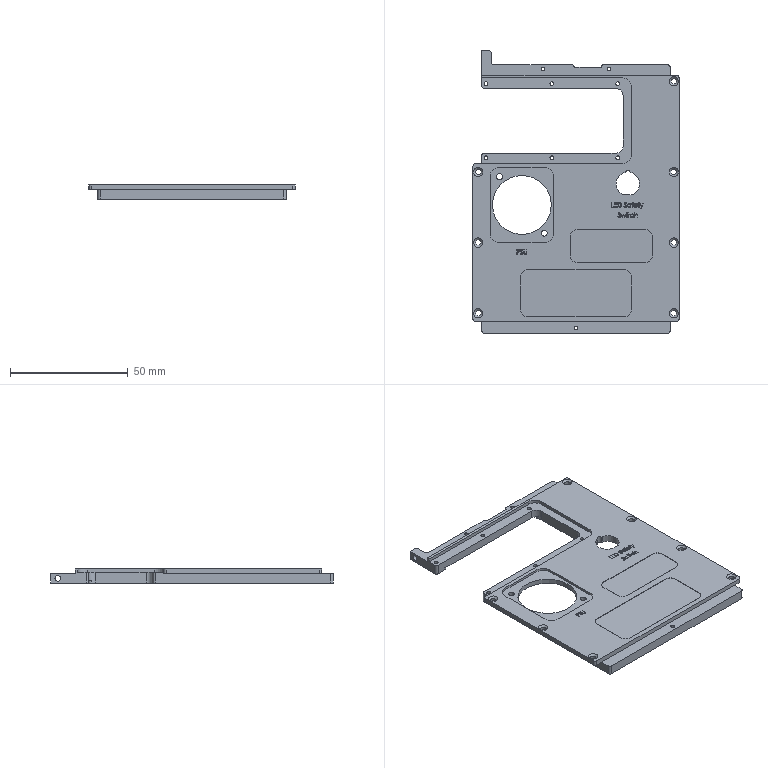NC program | NX | posted with a generic post | part box 87.5 x 120 x 6.001 mm
Lines 21 to 875 of 10039:
(ADAPTIVE_MILLING , TOOL : D6-18-D6-50-3T-ROUGH)
N40 T02 M6
N42 G53
N44 G17 G0 G90 X48.231 Y51.264 B0. C0. S6500 M3
N46 G43 Z50. H2
N48 Z-6.
N50 G94 G1 X48.234 Y51.239 Z-6.156 F3500.
N52 X48.237 Y51.214 Z-6.218
N54 X48.24 Y51.189 Z-6.263
N56 X48.243 Y51.164 Z-6.3
N58 X48.245 Y51.14 Z-6.331
N60 X48.248 Y51.115 Z-6.357
N62 X48.251 Y51.09 Z-6.38
N64 X48.254 Y51.065 Z-6.4
N66 X48.257 Y51.04 Z-6.418
N68 X48.26 Y51.015 Z-6.433
N70 X48.263 Y50.991 Z-6.447
N72 X48.266 Y50.966 Z-6.458
N74 X48.269 Y50.941 Z-6.468
N76 X48.272 Y50.916 Z-6.477
N78 X48.275 Y50.891 Z-6.484
N80 X48.277 Y50.866 Z-6.49
N82 X48.28 Y50.842 Z-6.494
N84 X48.283 Y50.817 Z-6.497
N86 X48.286 Y50.792 Z-6.499
N88 X48.289 Y50.767 Z-6.5
N90 X48.413 Y49.707
N92 G3 X48.692 Y49.265 R0.609
N94 X50.561 Y48.714 R4.722
N96 X56.014 Y48.464 R47.78
N98 G2 X60.858 Y48.431 R266.092
N100 X63.215 Y46.822 R3.486
N102 X64.391 Y43.389 R8.174
N104 X64.685 Y37.641 R45.423
N106 G1 X64.7 Y31.101
N108 X64.698 Y-44.39
N110 G2 X63.333 Y-46.758 R3.265
N112 X60.017 Y-48.071 R7.403
N114 X54.634 Y-48.425 R35.724
N116 G1 X46.714 Y-48.45
N118 X-60.638 Y-48.448
N120 G2 X-63.007 Y-47.073 R3.28
N122 X-64.322 Y-43.746 R7.447
N124 X-64.674 Y-38.363 R35.875
N126 G1 X-64.699 Y-30.563
N128 X-64.698 Y44.37
N130 G2 X-63.389 Y46.705 R3.246
N132 X-60.131 Y48.048 R7.217
N134 X-55.11 Y48.417 R32.115
N136 X-46.711 Y48.45 R653.142
N138 G1 X46.218 Y48.448
N140 G2 X49.506 Y48.064 R34.565
N142 G3 X56.918 Y47.67 R62.985
N144 G2 X59.184 Y47.6 R18.211
N146 X62.338 Y45.284 R4.681
N148 X63.573 Y41.358 R10.249
N150 X63.882 Y35.25 R51.582
N152 G1 X63.9 Y27.99
N154 X63.897 Y-42.368
N156 G2 X61.805 Y-45.898 R4.481
N158 X58.051 Y-47.25 R9.298
N160 X52.428 Y-47.62 R40.051
N162 G1 X44.388 Y-47.65
N164 X-58.572 Y-47.648
N166 G2 X-62.125 Y-45.582 R4.464
N168 X-63.511 Y-41.715 R9.344
N170 X-63.865 Y-36.271 R39.668
N172 X-63.899 Y-27.031 R690.714
N174 G1 Y42.288
N176 G2 X-61.821 Y45.884 R4.471
N178 X-58.004 Y47.256 R9.32
N180 X-52.501 Y47.616 R39.83
N182 G1 X-43.741 Y47.649
N184 X44.579 Y47.647
N186 G2 X49.672 Y47.237 R56.663
N188 G3 X57.232 Y46.862 R109.931
N190 G2 X61.401 Y44.156 R5.305
N192 X62.728 Y40.005 R11.071
N194 X63.078 Y33.659 R51.071
N196 G1 X63.1 Y26.399
N198 X63.099 Y-36.377
N200 X63.15 Y-36.998
N202 G2 X63.092 Y-41.028 R53.968
N204 X60.396 Y-45.143 R5.307
N206 X56.313 Y-46.466 R10.952
N208 X50.088 Y-46.825 R48.919
N210 G1 X42.168 Y-46.849
N212 X11.476 Y-46.85
N214 X10.999 Y-46.9
N216 X-54.442 Y-46.89
N218 G2 X-57.473 Y-46.816 R47.115
N220 X-61.37 Y-44.178 R5.29
N222 X-62.531 Y-41.145 R10.542
N224 X-63.065 Y-39.836 R4.344
N226 G1 X-63.15 Y-38.999
N228 X-63.145 Y39.222
N230 G2 X-63.008 Y41.628 R14.584
N232 X-60.283 Y45.21 R5.399
N234 X-56.24 Y46.475 R11.241
N236 G3 X-54.868 Y46.808 R4.797
N238 G1 X-54. Y46.9
N240 X48.501
N242 G2 X50.207 Y46.608 R9.102
N244 G3 X55.546 Y46.131 R38.286
N246 G2 X60.628 Y42.907 R5.952
N248 X61.938 Y38.495 R12.488
N250 X62.282 Y31.488 R60.228
N252 G1 X62.299 Y24.228
N254 X62.304 Y-34.388
N256 G3 X62.596 Y-34.928 R1.144
N258 G2 X63.1 Y-36.39 R4.185
N260 G1 X63.095 Y-36.33
N262 X62.934 Y-35.679
N264 G3 X62.596 Y-34.928 R4.351
N266 G2 X62.073 Y-33.687 R2.244
N268 X61.839 Y-29.756 R28.017
N270 G1 X61.819 Y-24.746
N272 X61.818 Y26.614
N274 G3 X61.664 Y35.971 R171.609
N276 X60.881 Y40.755 R19.457
N278 X58.658 Y44.117 R6.781
N280 X55.333 Y45.433 R7.527
N282 X51.211 Y45.987 R223.313
N284 G1 X50.951 Y46.099
N286 G3 X49.455 Y46.78 R4.647
N288 G2 X51.231 Y45.865 R4.245
N290 G3 X53.493 Y45.066 R7.668
N292 G2 X56.36 Y44.203 R14.581
N294 X59.706 Y40.547 R6.854
N296 X60.775 Y35.701 R16.143
N298 X61.013 Y27.607 R99.409
N300 G1 X61.019 Y21.967
N302 X61.02 Y-25.624
N304 G3 X61.162 Y-32.167 R87.18
N306 X61.393 Y-33.54 R6.272
N308 X62.085 Y-34.225 R3.54
N310 G1 X62.332 Y-34.565
N312 G3 X61.504 Y-33.7 R3.765
N314 G2 X61.02 Y-32.773 R1.83
N316 X60.61 Y-29.385 R15.183
N318 X60.539 Y-22.286 R254.423
N320 G1 X60.537 Y25.174
N322 G3 X60.373 Y34.351 R162.186
N324 X59.573 Y39.192 R19.888
N326 X56.631 Y43.154 R7.086
N328 X53.72 Y44.413 R13.134
N330 G2 X51.94 Y45.091 R12.871
N332 X51.597 Y45.512 R2.369
N334 G1 X51.108 Y45.956
N336 G2 X51.994 Y44.959 R3.712
N338 G3 X53.572 Y43.88 R5.597
N340 G2 X56.246 Y42.214 R13.059
N342 X58.804 Y38.005 R8.749
N344 X59.595 Y32.675 R23.4
N346 X59.738 Y22.838 R205.782
N348 G1 X59.739 Y-21.966
N350 G3 X59.86 Y-29.751 R139.122
N352 X60.412 Y-32.849 R10.652
N354 X60.689 Y-33.209 R0.809
N356 G1 X61.44 Y-33.643
N358 X60.577 Y-33.155
N360 G2 X59.845 Y-31.806 R2.823
N362 X59.35 Y-28.049 R16.534
N364 X59.259 Y-19.706 R223.119
N366 G1 X59.257 Y23.254
N368 G3 X59.084 Y32.851 R164.747
N370 X58.241 Y37.867 R20.503
N372 X56.79 Y40.656 R10.234
N374 G1 X56.739 Y40.801
N376 X56.245 Y41.587
N378 X55.587 Y42.245
N380 G3 X53.523 Y43.401 R20.997
N382 G2 X52.406 Y44.164 R4.996
N384 G1 X52.106 Y44.804
N386 X51.966 Y44.999
N388 G2 X52.344 Y44.26 R2.906
N390 G3 X53.26 Y43.142 R2.123
N392 X53.923 Y43.046 R6.592
N394 G1 X54.801 Y42.739
N396 X53.923 Y43.046
N398 G2 X53.122 Y43.167 R3.302
N400 X52.456 Y44.005 R0.968
N402 G3 X52.669 Y43.365 R1.378
N404 X53.27 Y43.12 R0.812
N406 G1 X53.923 Y43.046
N408 X54.801 Y42.739
N410 X55.587 Y42.245
N412 X56.245 Y41.587
N414 X56.739 Y40.801
N416 G2 X57.148 Y39.32 R5.513
N418 X58.384 Y29.657 R41.743
N420 X58.459 Y19.698 R459.539
N422 G1 X58.46 Y-21.064
N424 G3 X58.633 Y-28.817 R106.579
N426 X59.32 Y-32.159 R11.11
N428 X59.842 Y-32.921 R1.567
N430 G1 X60.689 Y-33.209
N432 X59.806 Y-32.924
N434 G2 X58.927 Y-31.785 R2.327
N436 X58.197 Y-28.457 R11.099
N438 X57.986 Y-21.796 R79.421
N440 G1 X57.979 Y-16.526
N442 Y36.514
N444 X57.98 Y36.547
N446 X58.083 Y38.365
N448 X58.118 Y38.845 Z-6.459
N450 G2 X58.584 Y39.302 Z-6.4 R0.606
N452 X59.297 Y38.797 R0.6 F15000.
N454 G1 X59.332 Y38.56
N456 X59.355 Y38.322
N458 G2 X58.633 Y37.756 R0.6
N460 X58.161 Y38.439 Z-6.478 R0.607 F3500.
N462 G1 X58.18 Y38.694 Z-6.5
N464 X58.261 Y39.767
N466 G3 X57.066 Y39.745 R-0.6
N468 G1 X57.15 Y38.999
N470 X57.157 Y10.899
N472 X57.179 Y2.619
N474 X57.18 Y-18.666
N476 G3 X57.348 Y-27.396 R136.933
N478 X58.09 Y-31.365 R14.301
N480 X58.95 Y-32.758 R3.687
N482 G1 X59.224 Y-32.874
N484 X59.863 Y-32.941
N486 G2 X58.964 Y-32.811 R3.687
N488 X57.86 Y-31.486 R2.814
N490 X57.15 Y-29.077 R9.496
N492 G1 Y-1.501
N494 X56.854 Y0.539
N496 G2 X56.704 Y5.446 R61.609
N498 G1 X56.696 Y9.702
N500 X57.034 Y10.587
N502 X57.15 Y11.499
N504 X57.034 Y10.587
N506 G2 X56.441 Y9.192 R40.775
N508 G3 X56.15 Y7.816 R9.32
N510 G1 X56.164 Y1.087
N512 X56.276 Y0.839
N514 X56.693 Y0.268
N516 X57.034 Y-0.587
N518 X56.693 Y0.268
N520 X56.276 Y0.839
N522 G2 X56.15 Y1.222 R0.665
N524 X56.166 Y8.856 R560.007
N526 X56.276 Y9.161 R0.851
N528 G1 X56.665 Y9.694
N530 G3 X56.197 Y9.012 R6.747
N532 X56.15 Y8.598 R1.645
N534 X56.407 Y8.105 R0.602
N536 G1 X56.662 Y7.928
N538 X57.624 Y7.259 Z-6.4
N540 X57.776 Y7.153 F15000.
N542 X57.906 Y7.02
N544 G2 X58.014 Y6.733 R0.64
N546 G1 X58.306 Y3.925
N548 X58.586 Y1.116
N550 G2 X58.934 Y-6.398 R88.816
N552 G1 X59.014 Y-27.212
N554 G2 X58.741 Y-27.718 R0.602
N556 G1 X58.623 Y-27.795
N558 X57.64 Y-28.433 Z-6.5 F3500.
N560 X57.345 Y-28.634
N562 G3 X57.15 Y-29.077 R0.605
N564 X57.191 Y-30.784 R11.965
N566 X58.2 Y-32.731 R3.335
N568 X58.535 Y-32.85 R1.13
N570 G1 X59.12 Y-32.863
N572 X58.415 Y-32.85
N574 G2 X57.456 Y-32.09 R1.629
N576 X57.15 Y-31.425 R1.686
N578 G1 Y-30.405
N580 X57.165 Y-31.843
N582 G3 X57.762 Y-32.788 R1.334
N584 X58.473 Y-32.85 R1.823
N586 G2 X57.738 Y-32.818 R2.723
N588 X57.15 Y-32.091 R0.951
N590 G1 Y-31.671
N592 G3 X57.172 Y-32.368 R13.47
N594 X57.98 Y-32.85 R0.711
N596 G2 X59.863 Y-32.941 R9.94
N598 X62.085 Y-34.225 R4.477
N600 G1 X62.596 Y-34.928
N602 G2 X62.934 Y-35.679 R4.351
N604 X63.15 Y-36.998 R4.495
N606 X63.121 Y-40.429 R56.537
N608 G1 X63.034 Y-40.847
N610 X62.669 Y-41.673
N612 G2 X57.098 Y-45.279 R9.596
N614 X51.509 Y-45.953 R27.376
N616 X40.41 Y-46.049 R341.091
N618 G1 X13.642 Y-46.053
N620 X13.418 Y-46.118
N622 G2 X11.868 Y-46.808 R4.677
N624 G1 X11.45 Y-46.852
N626 X11.868 Y-46.808
N628 G3 X13.5 Y-46.064 R4.808
N630 G2 X15.554 Y-45.685 R6.518
N632 X23.343 Y-45.569 R137.9
N634 G1 X43.443 Y-45.567
N636 G3 X52.62 Y-45.396 R154.11
N638 X57.687 Y-44.502 R19.437
N640 X60.288 Y-43.143 R10.269
N642 G2 X60.788 Y-43.05 R2.631
N644 G3 X62.166 Y-42.287 R3.662
N646 G2 X60.788 Y-43.05 R3.662
N648 G3 X58.112 Y-43.601 R14.811
N650 G2 X50.162 Y-44.672 R34.432
N652 X38.643 Y-44.769 R372.365
N654 G1 X22.226 Y-44.77
N656 G3 X15.809 Y-44.918 R82.244
N658 X14.414 Y-45.172 R4.888
N660 X14.097 Y-45.512 R1.186
N662 G1 X13.451 Y-46.099
N664 G3 X14.34 Y-45.182 R4.391
N666 G2 X15.957 Y-44.605 R3.761
N668 X20.792 Y-44.309 R32.801
N670 G1 X25.563 Y-44.289
N672 X41.583 Y-44.287
N674 G3 X51.72 Y-44.094 R167.09
N676 X57.841 Y-43.15 R34.625
N678 G1 X59.999
N680 X54.121
N682 G2 X41.49 Y-43.484 R181.661
N684 G1 X36.93 Y-43.489
N686 X24.626 Y-43.49
N688 G3 X17.719 Y-43.653 R91.021
N690 X15.006 Y-44.224 R8.614
N692 X14.606 Y-44.804 R1.055
N694 G1 X14.291 Y-45.242
N696 G3 X14.791 Y-44.381 R2.588
N698 G2 X15.973 Y-43.663 R2.371
N700 X19.584 Y-43.119 R14.315
N702 X26.884 Y-43.009 R160.409
N704 G1 X39.723 Y-43.007
N706 X44.02 Y-43.008
N708 G3 X44.997 Y-43.15 R2.845
N710 G1 X54.177
N712 X44.882 Y-43.148
N714 G2 X43.319 Y-42.795 R5.248
N716 G3 X40.388 Y-42.327 R10.952
N718 X31.281 Y-42.21 R186.605
N720 X20.46 Y-42.301 R291.363
N722 X17.504 Y-42.612 R17.656
N724 G2 X16.214 Y-43.091 R4.318
N726 G3 X15.15 Y-43.553 R2.533
N728 X14.956 Y-44.005 R0.867
N730 G1 X14.787 Y-44.389
N732 G3 X15.016 Y-43.71 R2.058
N734 G2 X15.688 Y-43.13 R1.073
N736 G1 X16.361 Y-43.06
N738 G3 X15.437 Y-43.177 R16.635
N740 X15.003 Y-43.774 R0.694
N742 G2 X15.17 Y-43.364 R0.824
N744 X15.596 Y-43.14 R0.696
N746 G3 X17.803 Y-42.447 R4.335
N748 G2 X20.506 Y-41.904 R9.013
N750 X27.605 Y-41.731 R97.498
N752 X39.377 Y-41.815 R355.937
N754 X42.244 Y-42.127 R16.477
N756 G3 X43.374 Y-42.818 R12.847
N758 G1 X42.534 Y-42.338
N760 G3 X40.954 Y-41.485 R3.086
N762 X36.954 Y-41.016 R19.258
N764 X22.147 Y-41.03 R257.397
N766 X18.927 Y-41.44 R14.877
N768 X18.58 Y-41.781 R0.993
N770 G1 X17.936 Y-42.36
N772 X17.676 Y-42.51
N774 G3 X18.775 Y-41.514 R3.554
N776 G2 X20.23 Y-40.904 R3.309
N778 X24.668 Y-40.5 R24.661
N780 X37.195 Y-40.564 R219.745
N782 X40.993 Y-41.109 R15.928
N784 X41.692 Y-41.47 R1.406
N786 G3 X42.266 Y-42.087 R2.592
N788 G2 X41.559 Y-41.269 R2.636
N790 G3 X39.955 Y-40.376 R3.533
N792 X35.84 Y-39.781 R17.814
N794 X23.256 Y-39.785 R145.835
N796 X19.768 Y-40.373 R12.961
N798 X19.265 Y-40.727 R0.871
N800 G2 X18.772 Y-41.519 R3.182
N802 G3 X19.349 Y-40.568 R4.184
N804 G2 X20.821 Y-39.798 R3.186
N806 X24.842 Y-39.271 R18.285
N808 X36.417 Y-39.362 R117.882
N810 X40.167 Y-40.06 R14.116
N812 X41.165 Y-40.614 R2.714
N814 G3 X41.56 Y-41.27 R8.46
N816 G2 X41.14 Y-40.49 R3.083
N818 G3 X39.608 Y-39.399 R3.214
N820 X35.701 Y-38.607 R14.015
N822 X23.729 Y-38.582 R85.658
N824 X20.371 Y-39.297 R11.492
N826 X19.599 Y-39.812 R1.641
N828 G1 X19.312 Y-40.632
N830 X19.593 Y-39.752
N832 G2 X20.851 Y-38.85 R2.721
N834 X24.416 Y-38.111 R12.482
N836 X35.88 Y-38.174 R74.25
N838 X39.713 Y-39.055 R12.83
N840 X40.914 Y-39.869 R3.193
N842 G1 X41.21 Y-40.637
N844 G3 X40.853 Y-39.633 R45.482
N846 X39.288 Y-38.382 R3.471
N848 X35.507 Y-37.444 R12.742
N850 X24.245 Y-37.378 R59.726
N852 X20.77 Y-38.224 R11.333
N854 X19.715 Y-38.972 R2.762
N856 G1 X19.631 Y-39.184
N858 X19.528 Y-39.957
N860 X19.66 Y-39.007
N862 G2 X20.804 Y-37.942 R2.468
N864 X24.18 Y-36.985 R10.144
N866 X32.363 Y-36.749 R50.589
N868 X37.677 Y-37.408 R25.735
N870 X40.439 Y-38.737 R6.625
N872 X40.894 Y-39.37 R1.327
N874 G1 X40.956 Y-39.907
N876 G3 X40.795 Y-38.918 R3.767
N878 X39.242 Y-37.444 R3.461
N880 X35.485 Y-36.312 R11.647
N882 X24.359 Y-36.223 R44.377
N884 X20.779 Y-37.285 R10.443
N886 X19.714 Y-38.183 R2.867
N888 G1 X19.65 Y-38.417
N890 X19.642 Y-39.105
N892 X19.65 Y-38.297
N894 G2 X20.472 Y-37.218 R1.997
N896 X23.495 Y-35.987 R7.807
N898 X29.528 Y-35.476 R29.768
N900 X36.455 Y-36.057 R33.73
N902 X39.828 Y-37.413 R9.077
N904 X40.825 Y-38.516 R2.76
N906 G1 X40.871 Y-39.178
N908 X40.832 Y-38.305
N910 G3 X39.677 Y-36.794 R2.916
N912 X36.154 Y-35.331 R9.302
N914 X28.91 Y-34.725 R32.438
N916 X23.11 Y-35.364 R24.805
N918 X20.146 Y-36.79 R7.173
N920 X19.653 Y-37.496 R1.27
N922 G1 X19.65 Y-38.305
N924 G2 X19.683 Y-37.265 R4.687
N926 X20.95 Y-35.909 R2.973
N928 X24.69 Y-34.636 R10.371
N930 X35.835 Y-34.829 R33.454
N932 X39.576 Y-36.305 R10.218
N934 X40.813 Y-37.65 R3.715
N936 X40.85 Y-38.426 R2.528
N938 G3 X40.814 Y-37.374 R5.174
N940 X39.521 Y-35.713 R3.351
N942 X35.731 Y-34.132 R10.121
N944 X24.393 Y-33.965 R30.581
N946 X20.67 Y-35.391 R9.872
N948 X19.699 Y-36.362 R3.154
N950 G1 X19.65 Y-36.566
N952 Y-37.406
N954 Y-36.446
N956 G2 X20.498 Y-35.231 R2.294
N958 X23.675 Y-33.737 R8.186
N960 X30.207 Y-33.092 R24.764
N962 X36.723 Y-33.965 R24.498
N964 X40.051 Y-35.728 R8.366
N966 X40.832 Y-36.804 R3.013
N968 G1 X40.85 Y-37.635
N970 G3 X40.818 Y-36.46 R7.08
N972 X39.564 Y-34.747 R3.405
N974 X35.736 Y-33.024 R10.076
N976 X24.369 Y-32.85 R27.35
N978 X20.664 Y-34.37 R9.946
N980 X19.695 Y-35.375 R3.223
N982 G1 X19.65 Y-35.565
N984 Y-36.465
N986 G2 X19.679 Y-35.312 R6.194
N988 X20.974 Y-33.832 R3.247
N990 X24.884 Y-32.339 R10.652
N992 X35.968 Y-32.655 R26.506
N994 X39.696 Y-34.417 R9.975
N996 X40.83 Y-35.828 R3.731
N998 X40.85 Y-36.726 R10.285
N1000 G3 X40.832 Y-35.532 R38.393
N1002 X39.571 Y-33.73 R3.464
N1004 X35.749 Y-31.918 R10.129
N1006 X24.229 Y-31.765 R25.111
N1008 X20.546 Y-33.414 R9.695
N1010 X19.696 Y-34.341 R3.276
N1012 G1 X19.65 Y-34.536
N1014 Y-35.496
N1016 Y-34.416
N1018 G2 X20.572 Y-33.086 R2.532
N1020 X24.102 Y-31.4 R9.046
N1022 X32.133 Y-30.862 R23.817
N1024 X37.833 Y-32.232 R17.632
N1026 X40.53 Y-34.278 R6.76
N1028 X40.85 Y-34.936 R1.562
N1030 G1 Y-35.656
N1032 G3 X40.831 Y-34.516 R20.118
N1034 X39.585 Y-32.697 R3.544
N1036 X35.719 Y-30.796 R10.231
N1038 X24.138 Y-30.672 R23.615
N1040 X20.496 Y-32.394 R9.604
N1042 X19.693 Y-33.299 R3.197
N1044 G1 X19.65 Y-33.485
N1046 Y-34.445
N1048 Y-33.365
N1050 G2 X20.584 Y-32.006 R2.605
N1052 X24.078 Y-30.289 R9.168
N1054 X32.45 Y-29.747 R22.78
N1056 X38.023 Y-31.244 R16.631
N1058 X40.591 Y-33.335 R6.599
N1060 X40.85 Y-33.91 R1.383
N1062 G1 Y-34.69
N1064 G3 X40.833 Y-33.491 R51.415
N1066 X39.6 Y-31.648 R3.578
N1068 X35.695 Y-29.674 R10.325
N1070 X24.151 Y-29.55 R22.636
N1072 X20.512 Y-31.304 R9.764
N1074 X19.69 Y-32.239 R3.185
N1076 G1 X19.65 Y-32.416
N1078 Y-33.376
N1080 Y-32.296
N1082 G2 X20.501 Y-31.001 R2.56
N1084 X23.899 Y-29.224 R8.876
N1086 X32.167 Y-28.574 R21.641
N1088 X37.97 Y-30.129 R16.77
N1090 X40.597 Y-32.293 R6.734
N1092 X40.85 Y-32.859 R1.453
N1094 G1 Y-33.639
N1096 G3 X40.811 Y-32.334 R6.822
N1098 X39.407 Y-30.407 R3.99
N1100 X35.161 Y-28.405 R11.249
N1102 X24.053 Y-28.46 R21.904
N1104 X20.404 Y-30.31 R9.59
N1106 X19.673 Y-31.21 R2.503
N1108 X19.65 Y-32.355 R8.524
N1110 G1 Y-31.215
N1112 G2 X20.503 Y-29.908 R2.574
N1114 X23.965 Y-28.085 R9.043
N1116 X32.704 Y-27.498 R21.282
N1118 X38.364 Y-29.247 R15.539
N1120 X40.704 Y-31.402 R6.211
N1122 X40.85 Y-31.797 R1.29
N1124 G1 Y-32.577
N1126 G3 X40.816 Y-31.287 R7.102
N1128 X39.462 Y-29.366 R3.941
N1130 X35.302 Y-27.321 R11.08
N1132 X24.006 Y-27.354 R21.313
N1134 X20.364 Y-29.254 R9.473
N1136 X19.673 Y-30.123 R2.428
N1138 X19.65 Y-31.266 R6.615
N1140 G1 Y-30.126
N1142 G2 X20.543 Y-28.774 R2.65
N1144 X24.146 Y-26.91 R9.346
N1146 X36.412 Y-27.247 R20.887
N1148 X40.017 Y-29.416 R9.468
N1150 X40.84 Y-30.641 R3.317
N1152 G1 X40.85 Y-31.551
N1154 G3 X40.817 Y-30.205 R8.379
N1156 X39.502 Y-28.305 R3.934
N1158 X35.343 Y-26.21 R11.011
N1160 X23.958 Y-26.248 R20.87
N1162 X20.394 Y-28.127 R9.546
N1164 X19.671 Y-29.032 R2.464
N1166 X19.65 Y-30.17 R8.387
N1168 G1 Y-29.03
N1170 G2 X20.581 Y-27.635 R2.706
N1172 X24.206 Y-25.77 R9.544
N1174 X36.457 Y-26.146 R20.518
N1176 X40.05 Y-28.357 R9.43
N1178 X40.833 Y-29.524 R3.706
N1180 G1 X40.85 Y-30.469
N1182 G3 X40.817 Y-29.118 R8.662
N1184 X39.458 Y-27.165 R4.006
N1186 X35.179 Y-25.04 R11.266
N1188 X23.908 Y-25.142 R20.544
N1190 X20.371 Y-27.041 R9.482
N1192 X19.685 Y-27.881 R2.891
N1194 G1 X19.65 Y-28.053
N1196 Y-29.073
N1198 X19.654 Y-27.873
N1200 G2 X20.758 Y-26.371 R3.097
N1202 X24.748 Y-24.494 R10.455
N1204 X36.398 Y-25.006 R20.364
N1206 X40.057 Y-27.265 R9.508
N1208 X40.835 Y-28.433 R3.637
N1210 G1 X40.85 Y-29.37
N1212 G3 X40.818 Y-28.022 R7.93
N1214 X39.49 Y-26.087 R3.994
N1216 X35.224 Y-23.928 R11.2
N1218 X23.858 Y-24.036 R20.277
N1220 X20.293 Y-26.003 R9.338
N1222 X19.672 Y-26.813 R2.301
N1224 X19.65 Y-27.953 R7.306
N1226 G1 Y-26.813
N1228 G2 X20.587 Y-25.408 R2.744
N1230 X24.323 Y-23.488 R9.736
N1232 X36.458 Y-23.908 R20.066
N1234 X40.035 Y-26.135 R9.555
N1236 X40.841 Y-27.355 R3.307
N1238 G1 X40.85 Y-28.259
N1240 G3 X40.816 Y-26.907 R8.224
N1242 X39.434 Y-24.927 R4.08
N1244 X35.116 Y-22.772 R11.408
N1246 X23.752 Y-22.949 R20.041
N1248 X20.313 Y-24.87 R9.296
N1250 X19.668 Y-25.715 R2.26
N1252 X19.65 Y-26.852 R19.118
N1254 G1 X19.654 Y-25.652
N1256 G2 X20.764 Y-24.137 R3.124
N1258 X24.86 Y-22.214 R10.616
N1260 X36.443 Y-22.781 R19.97
N1262 X40.083 Y-25.076 R9.496
N1264 X40.845 Y-26.274 R3.031
N1266 G1 X40.85 Y-27.161
N1268 G3 X40.817 Y-25.805 R8.663
N1270 X39.446 Y-23.822 R4.071
N1272 X35.163 Y-21.66 R11.356
N1274 X23.808 Y-21.806 R19.944
N1276 X20.256 Y-23.808 R9.27
N1278 X19.671 Y-24.587 R2.214
N1280 X19.65 Y-25.725 R7.885
N1282 G1 Y-24.585
N1284 G2 X20.503 Y-23.253 R2.649
N1286 X24.059 Y-21.32 R9.339
N1288 X36.599 Y-21.719 R19.674
N1290 X40.13 Y-24.016 R9.299
N1292 X40.843 Y-25.152 R3.068
N1294 G1 X40.85 Y-26.051
N1296 G3 X40.814 Y-24.684 R8.242
N1298 X39.515 Y-22.769 R4.002
N1300 X35.313 Y-20.579 R11.1
N1302 X23.756 Y-20.699 R19.797
N1304 X20.342 Y-22.611 R9.327
N1306 X19.683 Y-23.433 R2.828
N1308 X19.65 Y-24.619 R6.036
N1310 G2 X19.678 Y-23.341 R7.754
N1312 X20.954 Y-21.747 R3.538
N1314 X25.324 Y-19.847 R11.411
N1316 X36.447 Y-20.536 R19.78
N1318 X40.084 Y-22.848 R9.552
N1320 X40.839 Y-24.013 R3.404
N1322 G1 X40.85 Y-24.928
N1324 G3 X40.812 Y-23.557 R7.702
N1326 X39.402 Y-21.55 R4.163
N1328 X34.951 Y-19.349 R11.626
N1330 X23.703 Y-19.593 R19.701
N1332 X20.288 Y-21.54 R9.23
N1334 X19.671 Y-22.355 R2.328
N1336 X19.65 Y-23.493 R8.075
N1338 G1 Y-22.353
N1340 G2 X20.597 Y-20.926 R2.782
N1342 X24.303 Y-18.994 R9.796
N1344 X36.542 Y-19.449 R19.573
N1346 X40.103 Y-21.751 R9.443
N1348 X40.837 Y-22.892 R3.502
N1350 G1 X40.85 Y-23.815
N1352 G3 X40.816 Y-22.457 R8.58
N1354 X39.47 Y-20.488 R4.068
N1356 X35.155 Y-18.281 R11.347
N1358 X23.704 Y-18.468 R19.626
N1360 X20.197 Y-20.509 R9.126
N1362 X19.66 Y-21.279 R1.837
N1364 G1 X19.65 Y-22.369
N1366 Y-21.229
N1368 G2 X20.503 Y-19.892 R2.66
N1370 X24.121 Y-17.925 R9.431
N1372 X36.594 Y-18.345 R19.464
N1374 X40.092 Y-20.618 R9.447
N1376 X40.842 Y-21.794 R3.243
N1378 G1 X40.85 Y-22.694
N1380 G3 X40.814 Y-21.327 R8.096
N1382 X39.513 Y-19.406 R4.038
N1384 X35.307 Y-17.201 R11.143
N1386 X23.65 Y-17.362 R19.54
N1388 X20.257 Y-19.331 R9.087
N1390 X19.667 Y-20.128 R2.129
N1392 X19.65 Y-21.258 R36.771
N1394 G2 X19.678 Y-19.979 R7.768
N1396 X20.921 Y-18.407 R3.518
N1398 X25.176 Y-16.504 R11.23
N1400 X36.486 Y-17.178 R19.568
N1402 X40.081 Y-19.485 R9.551
N1404 X40.838 Y-20.653 R3.467
N1406 G1 X40.85 Y-21.571
N1408 G3 X40.817 Y-20.218 R8.642
N1410 X39.475 Y-18.249 R4.087
N1412 X35.101 Y-16.013 R11.394
N1414 X23.651 Y-16.236 R19.514
N1416 X20.218 Y-18.244 R9.074
N1418 X19.671 Y-18.992 R2.167
N1420 X19.65 Y-20.13 R8.745
N1422 G2 X19.678 Y-18.852 R7.448
N1424 X20.922 Y-17.282 R3.518
N1426 X25.28 Y-15.353 R11.318
N1428 X36.539 Y-16.074 R19.51
N1430 X40.103 Y-18.386 R9.473
N1432 X40.837 Y-19.531 R3.5
N1434 G1 X40.85 Y-20.453
N1436 G3 X40.816 Y-19.095 R8.652
N1438 X39.475 Y-17.124 R4.075
N1440 X35.151 Y-14.902 R11.36
N1442 X23.706 Y-15.091 R19.515
N1444 X20.226 Y-17.112 R9.166
N1446 X19.664 Y-17.895 R1.987
N1448 G1 X19.65 Y-19.005
N1450 Y-17.865
N1452 G2 X20.548 Y-16.478 R2.726
N1454 X24.169 Y-14.532 R9.593
N1456 X36.644 Y-14.991 R19.339
N1458 X40.094 Y-17.253 R9.4
N1460 X40.842 Y-18.431 R3.226
N1462 G1 X40.85 Y-19.331
N1464 G3 X40.814 Y-17.964 R8.234
N1466 X39.438 Y-15.966 R4.136
N1468 X35.048 Y-13.746 R11.53
N1470 X23.706 Y-13.966 R19.499
N1472 X20.235 Y-15.978 R9.179
N1474 X19.666 Y-16.76 R2.063
N1476 G1 X19.65 Y-17.884
N1478 G2 X19.676 Y-16.611 R8.297
N1480 X20.922 Y-15.033 R3.512
N1482 X25.281 Y-13.1 R11.334
N1484 X36.591 Y-13.843 R19.433
N1486 X40.116 Y-16.154 R9.384
N1488 X40.84 Y-17.297 R3.32
N1490 G1 X40.85 Y-18.205
N1492 G3 X40.816 Y-16.848 R8.65
N1494 X39.51 Y-14.908 R4.036
N1496 X35.201 Y-12.664 R11.243
N1498 X23.652 Y-12.859 R19.44
N1500 X20.198 Y-14.891 R9.05
N1502 X19.663 Y-15.65 R1.898
N1504 G1 X19.65 Y-16.754
N1506 Y-15.614
N1508 G2 X20.528 Y-14.247 R2.73
N1510 X24.17 Y-12.28 R9.567
N1512 X36.59 Y-12.717 R19.332
N1514 X40.171 Y-15.093 R9.309
N1516 X40.838 Y-16.166 R3.326
N1518 G1 X40.85 Y-17.082
N1520 G3 X40.816 Y-15.723 R8.611
N1522 X39.473 Y-13.749 R4.098
N1524 X35.098 Y-11.508 R11.411
N1526 X23.652 Y-11.733 R19.432
N1528 X20.22 Y-13.743 R9.096
N1530 X19.671 Y-14.493 R2.179
N1532 X19.65 Y-15.631 R8.478
N1534 G1 Y-14.491
N1536 G2 X20.597 Y-13.058 R2.793
N1538 X24.32 Y-11.108 R9.845
N1540 X36.643 Y-11.613 R19.311
N1542 X40.193 Y-13.994 R9.219
N1544 X40.847 Y-15.091 R2.758
N1546 G1 X40.85 Y-15.958
N1548 G3 X40.816 Y-14.597 R8.548
N1550 X39.473 Y-12.624 R4.087
N1552 X35.141 Y-10.395 R11.374
N1554 X23.707 Y-10.588 R19.45
N1556 X20.227 Y-12.611 R9.183
N1558 X19.664 Y-13.394 R1.999
N1560 G1 X19.65 Y-14.506
N1562 Y-13.366
N1564 G2 X20.548 Y-11.978 R2.729
N1566 X24.172 Y-10.028 R9.595
N1568 X36.643 Y-10.487 R19.277
N1570 X40.092 Y-12.753 R9.415
N1572 X40.841 Y-13.932 R3.268
N1574 G1 X40.85 Y-14.832
N1576 G3 X40.814 Y-13.465 R8.186
N1578 X39.436 Y-11.465 R4.146
N1580 X35.046 Y-9.241 R11.539
N1582 X23.707 Y-9.462 R19.447
N1584 X20.235 Y-11.477 R9.19
N1586 X19.666 Y-12.26 R2.068
N1588 G1 X19.65 Y-13.384
N1590 G2 X19.676 Y-12.111 R8.301
N1592 X20.923 Y-10.531 R3.516
N1594 X25.282 Y-8.595 R11.361
N1596 X36.59 Y-9.339 R19.386
N1598 X40.116 Y-11.653 R9.407
N1600 X40.84 Y-12.798 R3.336
N1602 G1 X40.85 Y-13.706
N1604 G3 X40.816 Y-12.348 R8.644
N1606 X39.509 Y-10.406 R4.043
N1608 X35.2 Y-8.159 R11.246
N1610 X23.653 Y-8.355 R19.404
N1612 X20.198 Y-10.39 R9.06
N1614 X19.663 Y-11.149 R1.899
N1616 G1 X19.65 Y-12.252
N1618 Y-11.112
N1620 G2 X20.598 Y-9.681 R2.802
N1622 X24.378 Y-7.712 R9.891
N1624 X36.59 Y-8.213 R19.316
N1626 X40.171 Y-10.592 R9.312
N1628 X40.838 Y-11.666 R3.336
N1630 G1 X40.85 Y-12.582
N1632 G3 X40.816 Y-11.223 R8.606
N1634 X39.472 Y-9.247 R4.104
N1636 X35.097 Y-7.003 R11.411
N1638 X23.653 Y-7.229 R19.399
N1640 X20.218 Y-9.243 R9.112
N1642 X19.671 Y-9.992 R2.166
N1644 X19.65 Y-11.13 R8.908
N1646 G2 X19.679 Y-9.852 R7.444
N1648 X20.923 Y-8.279 R3.528
N1650 X25.232 Y-6.355 R11.301
N1652 X36.541 Y-7.067 R19.395
N1654 X40.1 Y-9.385 R9.496
N1656 X40.837 Y-10.531 R3.582
N1658 G1 X40.85 Y-11.457
N1660 G3 X40.816 Y-10.096 R8.588
N1662 X39.472 Y-8.12 R4.089
N1664 X35.097 Y-5.876 R11.413
N1666 X23.653 Y-6.103 R19.396
N1668 X20.226 Y-8.11 R9.14
N1670 X19.664 Y-8.894 R1.989
N1672 G1 X19.65 Y-10.004
N1674 Y-8.864
N1676 G2 X20.497 Y-7.525 R2.661
N1678 X24.122 Y-5.54 R9.433
N1680 X36.642 Y-5.982 R19.248
N1682 X40.093 Y-8.251 R9.407
N1684 X40.842 Y-9.431 R3.256
N1686 G1 X40.85 Y-10.33
N1688 G3 X40.814 Y-8.963 R8.245
N1690 X39.465 Y-6.988 R4.121
N1692 X35.148 Y-4.765 R11.379
N1694 X23.707 Y-4.958 R19.427
N1696 X20.234 Y-6.976 R9.204
N1698 X19.666 Y-7.759 R2.056
N1700 G1 X19.65 Y-8.881
N1702 G2 X19.676 Y-7.609 R8.437
N1704 X20.924 Y-6.027 R3.517
N1706 X25.232 Y-4.102 R11.295
N1708 X36.595 Y-4.837 R19.358
N1710 X40.117 Y-7.153 R9.417
N1712 X40.84 Y-8.297 R3.315
N1714 G1 X40.85 Y-9.204
N1716 G3 X40.82 Y-7.861 R8.716
N1718 X39.508 Y-5.902 R4.034
N1720 X35.25 Y-3.67 R11.205
N1722 X23.707 Y-3.831 R19.416
N1724 X20.277 Y-5.807 R9.286
N1726 X19.678 Y-6.588 R2.514
N1728 X19.65 Y-7.75 R6.944
N1730 G1 Y-6.61
N1732 G2 X20.599 Y-5.177 R2.809
N1734 X24.359 Y-3.213 R9.885
N1736 X36.589 Y-3.709 R19.299
N1738 X40.11 Y-6.019 R9.458
N1740 X40.839 Y-7.164 R3.385
N1742 G1 X40.85 Y-8.077